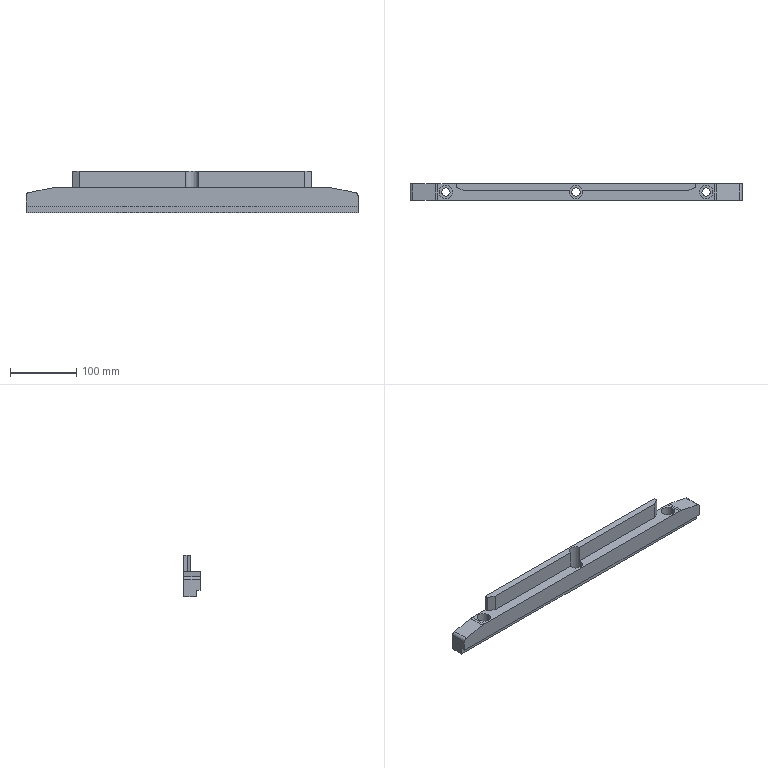NC program | NX | posted with a generic post | part box 500 x 25 x 62.5 mm
Lines 1 to 1034 of 5890:
N10 G17 G21 G94 G90
(ADAPTIVE_MILLING , TOOL : D12JING)
N12 T21 M6
N14 G54
N16 G17 G0 G90 X188.999 Y20.604 S9500 M3
N18 G43 Z30. H21
N20 Z-23.849
N22 G94 G1 Z-24.849 F1000.
N24 X186.723 Y19.599 F3000.
N26 G3 X186. Y18.491 R1.224
N28 G2 X189.082 Y12.674 R11.639
N30 X189.893 Y4.779 R39.403
N32 X189.954 Y-9.769 R368.863
N34 X186.791 Y-14.661 R7.16
N36 X180.65 Y-16.914 R14.438
N38 X172.048 Y-17.442 R63.898
N40 G1 X170.998 Y-17.454
N42 X169.798 Y-17.465
N44 X168.298 Y-17.473
N46 X166.348 Y-17.48
N48 X163.573 Y-17.484
N50 X158.623 Y-17.487
N52 X129.898 Y-17.488
N54 X21.673
N56 X20.923 Y-17.492
N58 X20.023 Y-17.493
N60 X19.573
N62 X18.748 Y-17.496
N64 X17.548 Y-17.495
N66 X16.873 Y-17.497
N68 X15.673 Y-17.496
N70 X14.698 Y-17.499
N72 X13.948 Y-17.498
N74 X12.598 Y-17.5
N76 X12.148 Y-17.501
N78 X11.323 Y-17.499
N80 X10.198 Y-17.501
N82 X9.448 Y-17.499
N84 X8.248 Y-17.501
N86 X7.348 Y-17.499
N88 X6.598 Y-17.5
N90 X5.323 Y-17.498
N92 X4.873
N94 X4.048 Y-17.5
N96 X2.923 Y-17.498
N98 X2.173 Y-17.499
N100 X0.898 Y-17.498
N102 X0.148 Y-17.499
N104 X-1.202 Y-17.497
N106 X-1.877 Y-17.498
N108 X-3.152 Y-17.497
N110 X-3.677
N112 X-4.502 Y-17.499
N114 X-5.702 Y-17.497
N116 X-6.602 Y-17.5
N118 X-7.652 Y-17.497
N120 X-8.477 Y-17.499
N122 X-9.677 Y-17.498
N124 X-10.652 Y-17.5
N126 X-11.627 Y-17.498
N128 X-12.452 Y-17.5
N130 X-13.652 Y-17.498
N132 X-14.327 Y-17.499
N134 X-15.527 Y-17.498
N136 X-16.577 Y-17.501
N138 X-17.477 Y-17.499
N140 X-18.602 Y-17.501
N142 X-19.352 Y-17.499
N144 X-20.552 Y-17.501
N146 X-21.452 Y-17.499
N148 X-22.202 Y-17.5
N150 X-23.477 Y-17.498
N152 X-24.002 Y-17.497
N154 X-24.752 Y-17.499
N156 X-25.952 Y-17.498
N158 X-26.927 Y-17.5
N160 X-27.901 Y-17.498
N162 X-28.726 Y-17.5
N164 X-29.926 Y-17.498
N166 X-30.601 Y-17.499
N168 X-31.801 Y-17.498
N170 X-32.851 Y-17.501
N172 X-33.751 Y-17.499
N174 X-34.876 Y-17.501
N176 X-35.626 Y-17.499
N178 X-36.826 Y-17.501
N180 X-37.726 Y-17.499
N182 X-38.476 Y-17.5
N184 X-39.751 Y-17.498
N186 X-40.276 Y-17.497
N188 X-41.026 Y-17.499
N190 X-42.226 Y-17.498
N192 X-43.201 Y-17.5
N194 X-44.176 Y-17.498
N196 X-45.001 Y-17.5
N198 X-46.201 Y-17.498
N200 X-46.876 Y-17.499
N202 X-48.076 Y-17.498
N204 X-49.126 Y-17.501
N206 X-50.026 Y-17.499
N208 X-51.151 Y-17.501
N210 X-51.901 Y-17.499
N212 X-53.101 Y-17.501
N214 X-54.001 Y-17.499
N216 X-54.751 Y-17.5
N218 X-56.026 Y-17.498
N220 X-56.551 Y-17.497
N222 X-57.301 Y-17.499
N224 X-58.501 Y-17.498
N226 X-59.176 Y-17.499
N228 X-60.301 Y-17.498
N230 X-61.426 Y-17.5
N232 X-62.626 Y-17.497
N234 X-63.301 Y-17.499
N236 X-64.576 Y-17.498
N238 X-65.026 Y-17.497
N240 X-65.776 Y-17.499
N242 X-66.751 Y-17.498
N244 X-67.576 Y-17.5
N246 X-68.701 Y-17.498
N248 X-69.601 Y-17.5
N250 X-70.651 Y-17.498
N252 X-71.326 Y-17.499
N254 X-72.301 Y-17.498
N256 X-72.676
N258 X-73.351 Y-17.499
N260 X-74.401 Y-17.498
N262 X-74.926
N264 X-75.451 Y-17.499
N266 X-76.351 Y-17.498
N268 X-76.726 Y-17.497
N270 X-77.401 Y-17.499
N272 X-78.451 Y-17.498
N274 X-78.901 Y-17.497
N276 X-79.576 Y-17.499
N278 X-80.551 Y-17.498
N280 X-81.076
N282 X-81.751 Y-17.499
N284 X-82.801 Y-17.497
N286 X-83.776 Y-17.5
N288 X-84.676 Y-17.498
N290 X-85.501 Y-17.5
N292 X-86.476 Y-17.498
N294 X-87.301 Y-17.5
N296 X-88.276 Y-17.499
N298 X-88.951 Y-17.5
N300 X-90.226 Y-17.498
N302 X-91.051 Y-17.5
N304 X-92.101 Y-17.498
N306 X-93.076 Y-17.501
N308 X-94.051 Y-17.499
N310 X-94.876 Y-17.5
N312 X-96.076 Y-17.498
N314 X-96.826 Y-17.5
N316 X-97.801 Y-17.499
N318 X-98.851 Y-17.501
N320 X-99.676 Y-17.499
N322 X-100.801 Y-17.501
N324 X-101.626 Y-17.499
N326 X-102.751 Y-17.501
N328 X-103.576 Y-17.499
N330 X-104.476 Y-17.5
N332 X-105.526 Y-17.499
N334 X-106.426 Y-17.501
N336 X-107.476 Y-17.498
N338 X-108.301 Y-17.5
N340 X-109.426 Y-17.498
N342 X-110.176 Y-17.5
N344 X-111.226 Y-17.498
N346 X-112.201 Y-17.5
N348 X-112.876 Y-17.499
N350 X-114.151 Y-17.501
N352 X-114.601 Y-17.502
N354 X-115.351 Y-17.5
N356 X-116.551 Y-17.501
N358 X-117.526 Y-17.499
N360 X-118.501 Y-17.501
N362 X-119.326 Y-17.499
N364 X-120.526 Y-17.501
N366 X-121.201 Y-17.5
N368 X-122.401 Y-17.501
N370 X-123.151 Y-17.5
N372 X-124.351 Y-17.501
N374 X-125.026 Y-17.5
N376 X-126.001 Y-17.501
N378 X-126.451 Y-17.502
N380 X-127.276 Y-17.5
N382 X-128.176 Y-17.501
N384 X-129.001 Y-17.5
N386 X-130.201 Y-17.501
N388 X-130.951 Y-17.5
N390 X-131.926 Y-17.501
N392 X-132.751 Y-17.499
N394 X-133.876 Y-17.501
N396 X-134.701 Y-17.499
N398 X-135.676 Y-17.501
N400 X-136.501 Y-17.499
N402 X-137.551 Y-17.501
N404 X-138.451 Y-17.499
N406 X-139.501 Y-17.501
N408 X-140.326 Y-17.499
N410 X-141.526 Y-17.501
N412 X-142.576 Y-17.498
N414 X-143.401 Y-17.5
N416 X-144.601 Y-17.498
N418 X-145.576 Y-17.501
N420 X-146.476 Y-17.499
N422 X-147.676 Y-17.501
N424 X-148.576 Y-17.499
N426 X-149.551 Y-17.501
N428 X-150.526 Y-17.499
N430 X-151.576 Y-17.501
N432 X-152.401 Y-17.499
N434 X-153.526 Y-17.501
N436 X-154.351 Y-17.499
N438 X-155.476 Y-17.501
N440 X-156.301 Y-17.499
N442 X-157.201 Y-17.5
N444 X-158.026 Y-17.499
N446 X-159.151 Y-17.501
N448 X-160.051 Y-17.499
N450 X-160.951 Y-17.501
N452 X-161.776 Y-17.499
N454 X-162.751 Y-17.5
N456 X-163.801 Y-17.498
N458 X-164.701 Y-17.5
N460 X-165.601 Y-17.499
N462 X-166.501 Y-17.5
N464 X-167.476 Y-17.498
N466 X-168.151 Y-17.499
N468 X-169.426 Y-17.498
N470 X-169.951
N472 X-170.551 Y-17.499
N474 X-171.526 Y-17.498
N476 X-172.276 Y-17.5
N478 X-173.326 Y-17.498
N480 X-174.301 Y-17.5
N482 X-174.976 Y-17.499
N484 X-176.251 Y-17.501
N486 X-176.776
N488 G2 X-182.25 Y-17.469 R279.255
N490 X-187.15 Y-14.319 R7.147
N492 X-189.421 Y-8.106 R14.464
N494 X-189.954 Y1.471 R71.167
N496 X-189.956 Y9.795 R359.357
N498 X-187.917 Y14.399 R9.324
N500 G3 X-186.115 Y16.886 R22.32
N502 G1 X-186.089 Y16.956
N504 X-186.067 Y17.028
N506 X-186.048 Y17.1
N508 X-186.034 Y17.174
N510 X-186.024 Y17.248
N512 X-186.328 Y18.409
N514 G3 X-187.009 Y19.204 R1.217
N516 X-188.412 Y18.879 Z-24.785 R1.228
N518 G1 X-189.02 Y18.273 Z-24.749
N520 X-189.418 Y17.87
N522 X-189.833 Y17.485
N524 G2 X-191.728 Y18.409 R1.202
N526 G1 X-191.757 Y18.961
N528 X-191.76 Y19.514
N530 G2 X-190.268 Y20.526 R1.204
N532 G1 X-189.229 Y20.257
N534 X-186.906 Y19.653 Z-24.849
N536 G2 X-186.368 Y19.311 R1.26
N538 X-186.018 Y18.462 R1.291
N540 X-186.092 Y16.745 R6.843
N542 X-187.495 Y14.099 R19.023
N544 G3 X-189.115 Y7.901 R16.064
N546 X-188.942 Y-6.48 R85.448
N548 X-187.347 Y-11.993 R14.997
N550 X-182.305 Y-15.789 R8.996
N552 X-175.501 Y-16.787 R24.761
N554 X-155.402 Y-16.9 R819.463
N556 G1 X-153.827 Y-16.902
N558 X-153.152
N560 X-152.777 Y-16.901
N562 X-151.877 Y-16.902
N564 X-151.277 Y-16.9
N566 X-150.002 Y-16.902
N568 X-149.327 Y-16.9
N570 X-147.752 Y-16.902
N572 X-146.777 Y-16.9
N574 X-146.102 Y-16.901
N576 X-144.977 Y-16.899
N578 X-144.152 Y-16.901
N580 X-142.652 Y-16.898
N582 X-141.902 Y-16.9
N584 X-141.152 Y-16.898
N586 X-139.577 Y-16.901
N588 X-139.127
N590 X-138.002 Y-16.902
N592 X-137.477 Y-16.901
N594 X-136.427 Y-16.899
N596 X-135.977 Y-16.9
N598 X-135.602 Y-16.899
N600 X-134.102 Y-16.902
N602 X-133.577
N604 X-132.452 Y-16.903
N606 X-131.927 Y-16.902
N608 X-128.852 Y-16.898
N610 X-126.377
N612 X-124.352 Y-16.901
N614 X-123.827
N616 X-122.852 Y-16.903
N618 X-122.327 Y-16.901
N620 X-120.602 Y-16.903
N622 X-120.152 Y-16.902
N624 X-118.727 Y-16.904
N626 X-118.277 Y-16.903
N628 X-117.902
N630 X-117.602 Y-16.902
N632 X-116.852 Y-16.903
N634 X-116.327 Y-16.902
N636 X-115.502 Y-16.903
N638 X-114.902 Y-16.902
N640 X-114.452
N642 X-113.777 Y-16.9
N644 X-113.027 Y-16.901
N646 X-111.902 Y-16.898
N648 X-110.477 Y-16.901
N650 X-110.027 Y-16.9
N652 X-108.827 Y-16.902
N654 X-108.152 Y-16.9
N656 X-107.177 Y-16.901
N658 X-106.127 Y-16.899
N660 X-105.527 Y-16.9
N662 X-104.027 Y-16.898
N664 X-103.127 Y-16.9
N666 X-102.002 Y-16.898
N668 X-101.252 Y-16.9
N670 X-100.652 Y-16.899
N672 X-99.602 Y-16.901
N674 X-98.402 Y-16.898
N676 X-97.877 Y-16.899
N678 X-96.452 Y-16.897
N680 X-95.477 Y-16.899
N682 X-94.577 Y-16.897
N684 X-94.052 Y-16.898
N686 X-92.327 Y-16.896
N688 X-91.652 Y-16.898
N690 X-90.377 Y-16.896
N692 X-89.777 Y-16.898
N694 X-88.952 Y-16.897
N696 X-87.902 Y-16.899
N698 X-86.852 Y-16.897
N700 X-86.027 Y-16.899
N702 X-85.352 Y-16.897
N704 X-84.602 Y-16.899
N706 X-83.102 Y-16.896
N708 X-82.202 Y-16.899
N710 X-81.602 Y-16.897
N712 X-80.027 Y-16.9
N714 X-79.052 Y-16.898
N716 X-77.627 Y-16.9
N718 X-77.102 Y-16.899
N720 X-76.352 Y-16.901
N722 X-75.153 Y-16.898
N724 X-74.628 Y-16.899
N726 X-74.028 Y-16.897
N728 X-73.503 Y-16.898
N730 X-72.828 Y-16.897
N732 X-72.003 Y-16.899
N734 X-71.328 Y-16.898
N736 X-69.753 Y-16.9
N738 X-69.303 Y-16.899
N740 X-68.553 Y-16.901
N742 X-67.278 Y-16.898
N744 X-65.703 Y-16.9
N746 X-65.253 Y-16.899
N748 X-64.128 Y-16.901
N750 X-62.853 Y-16.898
N752 X-61.503 Y-16.9
N754 X-60.978 Y-16.899
N756 X-60.303 Y-16.9
N758 X-59.853 Y-16.899
N760 X-59.478 Y-16.9
N762 X-58.878 Y-16.899
N764 X-57.678 Y-16.901
N766 X-56.628 Y-16.898
N768 X-55.878 Y-16.9
N770 X-54.303 Y-16.898
N772 X-53.478 Y-16.9
N774 X-52.278 Y-16.898
N776 X-51.528 Y-16.9
N778 X-50.628 Y-16.898
N780 X-49.203 Y-16.9
N782 X-48.753
N784 X-47.853 Y-16.901
N786 X-46.653 Y-16.898
N788 X-45.828 Y-16.9
N790 X-45.003 Y-16.898
N792 X-43.353 Y-16.901
N794 X-42.903 Y-16.899
N796 X-41.778 Y-16.901
N798 X-41.328 Y-16.9
N800 X-40.578 Y-16.901
N802 X-39.153 Y-16.903
N804 X-38.628 Y-16.901
N806 X-37.803 Y-16.9
N808 X-37.353
N810 X-36.678 Y-16.899
N812 X-35.328 Y-16.902
N814 X-34.578 Y-16.899
N816 X-32.853 Y-16.902
N818 X-32.403 Y-16.901
N820 X-31.128 Y-16.902
N822 X-30.678 Y-16.901
N824 X-29.928 Y-16.9
N826 X-29.328 Y-16.901
N828 X-28.653 Y-16.899
N830 X-27.003 Y-16.901
N832 X-26.103 Y-16.899
N834 X-25.428 Y-16.9
N836 X-24.903 Y-16.899
N838 X-24.303 Y-16.9
N840 X-22.878 Y-16.902
N842 X-22.503 Y-16.901
N844 X-21.828 Y-16.902
N846 X-21.378 Y-16.901
N848 X-20.928 Y-16.902
N850 X-20.253 Y-16.9
N852 X-18.678 Y-16.902
N854 X-16.878 Y-16.903
N856 X-15.903 Y-16.9
N858 X-15.003 Y-16.902
N860 X-13.803 Y-16.899
N862 X-13.053 Y-16.9
N864 X-12.078 Y-16.898
N866 X-11.403 Y-16.9
N868 X-10.053 Y-16.897
N870 X-9.528 Y-16.898
N872 X-7.728 Y-16.895
N874 X-6.903 Y-16.898
N876 X-6.078 Y-16.896
N878 X-4.653 Y-16.899
N880 X-3.528 Y-16.897
N882 X-2.103 Y-16.9
N884 X-1.428 Y-16.898
N886 X-0.828 Y-16.899
N888 X0.522 Y-16.897
N890 X1.797 Y-16.899
N892 X2.397 Y-16.898
N894 X3.147 Y-16.9
N896 X3.597 Y-16.899
N898 X4.347 Y-16.9
N900 X4.797
N902 X5.922 Y-16.902
N904 X6.597 Y-16.9
N906 X8.097 Y-16.902
N908 X9.897 Y-16.904
N910 X11.097 Y-16.9
N912 X12.372 Y-16.902
N914 X12.897 Y-16.901
N916 X13.647 Y-16.899
N918 X14.022 Y-16.9
N920 X15.372 Y-16.896
N922 X15.897 Y-16.897
N924 X18.072 Y-16.892
N926 X18.672 Y-16.893
N928 X19.497 Y-16.89
N930 X20.997 Y-16.892
N932 X21.522 Y-16.89
N934 X23.022 Y-16.892
N936 X23.622 Y-16.89
N938 X24.522 Y-16.888
N940 X25.347 Y-16.89
N942 X26.022 Y-16.888
N944 X26.847 Y-16.89
N946 X27.447 Y-16.888
N948 X28.272 Y-16.89
N950 X28.872 Y-16.888
N952 X29.622 Y-16.89
N954 X30.222 Y-16.888
N956 X31.047 Y-16.89
N958 X31.647 Y-16.888
N960 X32.397 Y-16.89
N962 X32.997 Y-16.888
N964 X33.822 Y-16.89
N966 X34.422 Y-16.888
N968 X35.172 Y-16.89
N970 X35.772 Y-16.888
N972 X36.597 Y-16.89
N974 X37.197 Y-16.888
N976 X37.947 Y-16.89
N978 X38.547 Y-16.888
N980 X39.372 Y-16.89
N982 X40.047 Y-16.888
N984 X40.872 Y-16.89
N986 X41.472 Y-16.888
N988 X42.297 Y-16.89
N990 X42.897 Y-16.888
N992 X43.647 Y-16.89
N994 X44.247 Y-16.888
N996 X45.072 Y-16.89
N998 X45.672 Y-16.888
N1000 X46.422 Y-16.89
N1002 X47.022 Y-16.888
N1004 X47.847 Y-16.89
N1006 X48.447 Y-16.888
N1008 X49.197 Y-16.89
N1010 X49.797 Y-16.888
N1012 X50.622 Y-16.89
N1014 X51.222 Y-16.888
N1016 X51.972 Y-16.89
N1018 X52.572 Y-16.888
N1020 X53.397 Y-16.89
N1022 X53.997 Y-16.888
N1024 X54.747 Y-16.89
N1026 X55.347 Y-16.888
N1028 X56.172 Y-16.89
N1030 X56.847 Y-16.888
N1032 X57.672 Y-16.89
N1034 X58.272 Y-16.888
N1036 X59.097 Y-16.89
N1038 X59.697 Y-16.888
N1040 X60.447 Y-16.89
N1042 X61.047 Y-16.888
N1044 X61.872 Y-16.89
N1046 X62.472 Y-16.888
N1048 X63.222 Y-16.89
N1050 X63.822 Y-16.888
N1052 X64.647 Y-16.89
N1054 X65.247 Y-16.888
N1056 X65.997 Y-16.89
N1058 X66.597 Y-16.888
N1060 X67.422 Y-16.89
N1062 X68.022 Y-16.888
N1064 X68.772 Y-16.89
N1066 X69.372 Y-16.888
N1068 X70.197 Y-16.89
N1070 X70.797 Y-16.888
N1072 X71.547 Y-16.89
N1074 X72.147 Y-16.888
N1076 X72.972 Y-16.89
N1078 X73.647 Y-16.888
N1080 X74.472 Y-16.89
N1082 X75.072 Y-16.888
N1084 X75.897 Y-16.89
N1086 X76.497 Y-16.888
N1088 X77.247 Y-16.89
N1090 X77.847 Y-16.888
N1092 X78.672 Y-16.89
N1094 X79.272 Y-16.888
N1096 X80.022 Y-16.89
N1098 X80.622 Y-16.888
N1100 X81.447 Y-16.89
N1102 X82.047 Y-16.888
N1104 X82.797 Y-16.89
N1106 X83.397 Y-16.888
N1108 X84.222 Y-16.89
N1110 X84.897 Y-16.888
N1112 X85.797 Y-16.89
N1114 X86.472 Y-16.888
N1116 X87.297 Y-16.89
N1118 X87.897 Y-16.888
N1120 X88.722 Y-16.89
N1122 X89.397 Y-16.888
N1124 X90.297 Y-16.89
N1126 X90.972 Y-16.888
N1128 X91.797 Y-16.89
N1130 X92.397 Y-16.888
N1132 X93.222 Y-16.89
N1134 X93.897 Y-16.888
N1136 X94.797 Y-16.89
N1138 X95.472 Y-16.888
N1140 X96.297 Y-16.89
N1142 X96.897 Y-16.888
N1144 X97.722 Y-16.89
N1146 X98.397 Y-16.888
N1148 X99.297 Y-16.89
N1150 X99.972 Y-16.888
N1152 X100.797 Y-16.89
N1154 X101.397 Y-16.888
N1156 X102.222 Y-16.89
N1158 X102.897 Y-16.888
N1160 X103.797 Y-16.89
N1162 X104.472 Y-16.888
N1164 X105.297 Y-16.89
N1166 X105.897 Y-16.888
N1168 X106.722 Y-16.89
N1170 X107.397 Y-16.888
N1172 X108.297 Y-16.89
N1174 X108.972 Y-16.888
N1176 X109.797 Y-16.89
N1178 X110.397 Y-16.888
N1180 X111.222 Y-16.89
N1182 X111.897 Y-16.888
N1184 X112.797 Y-16.89
N1186 X113.472 Y-16.888
N1188 X114.372 Y-16.89
N1190 X115.047 Y-16.888
N1192 X115.872 Y-16.89
N1194 X116.472 Y-16.888
N1196 X117.297 Y-16.89
N1198 X117.972 Y-16.888
N1200 X118.872 Y-16.89
N1202 X119.547 Y-16.888
N1204 X120.372 Y-16.89
N1206 X120.972 Y-16.888
N1208 X121.797 Y-16.89
N1210 X122.472 Y-16.888
N1212 X123.372 Y-16.89
N1214 X124.047 Y-16.888
N1216 X124.872 Y-16.89
N1218 X125.472 Y-16.888
N1220 X126.297 Y-16.89
N1222 X126.972 Y-16.888
N1224 X127.872 Y-16.89
N1226 X128.547 Y-16.888
N1228 X129.372 Y-16.89
N1230 X129.972 Y-16.888
N1232 X130.797 Y-16.89
N1234 X131.472 Y-16.888
N1236 X132.372 Y-16.89
N1238 X133.047 Y-16.888
N1240 X133.872 Y-16.89
N1242 X134.472 Y-16.888
N1244 X135.297 Y-16.89
N1246 X135.972 Y-16.888
N1248 X136.872 Y-16.89
N1250 X137.547 Y-16.888
N1252 X138.372 Y-16.89
N1254 X138.972 Y-16.888
N1256 X139.797 Y-16.89
N1258 X140.472 Y-16.888
N1260 X141.372 Y-16.89
N1262 X142.047 Y-16.888
N1264 X142.872 Y-16.89
N1266 X143.472 Y-16.888
N1268 X144.297 Y-16.89
N1270 X144.972 Y-16.888
N1272 X145.872 Y-16.89
N1274 X146.547 Y-16.888
N1276 X147.372 Y-16.89
N1278 X148.047 Y-16.888
N1280 X148.947 Y-16.89
N1282 X149.622 Y-16.888
N1284 X150.447 Y-16.889
N1286 X151.122 Y-16.888
N1288 X151.947 Y-16.889
N1290 X152.622 Y-16.888
N1292 X153.447 Y-16.889
N1294 X154.122 Y-16.888
N1296 X154.947 Y-16.889
N1298 X155.697 Y-16.887
N1300 X156.447 Y-16.889
N1302 X157.197 Y-16.887
N1304 X157.947 Y-16.888
N1306 X158.772 Y-16.886
N1308 X159.447 Y-16.888
N1310 X160.497 Y-16.885
N1312 X161.097 Y-16.886
N1314 X162.897 Y-16.882
N1316 X163.497
N1318 X164.247
N1320 X165.297 Y-16.881
N1322 X166.422 Y-16.88
N1324 G3 X177.814 Y-16.568 R149.249
N1326 X183.919 Y-15.143 R18.297
N1328 X188.11 Y-10.259 R8.557
N1330 X189.221 Y-3.931 R21.167
N1332 X188.969 Y9.106 R92.609
N1334 X186.487 Y16.423 R16.369
N1336 G2 X186.01 Y17.518 R4.405
N1338 G1 X186.364 Y18.664
N1340 G2 X186.969 Y19.381 R1.229
N1342 X188.44 Y19.077 Z-24.782 R1.224
N1344 G1 X188.991 Y18.523 Z-24.749
N1346 X189.42 Y18.084
N1348 X189.868 Y17.664
N1350 G3 X191.764 Y18.664 R1.202
N1352 G1 X191.757 Y19.099
N1354 X191.732 Y19.533
N1356 G3 X190.275 Y20.485 R1.205
N1358 G1 X189.224 Y20.236
N1360 X186.889 Y19.681 Z-24.849
N1362 G3 X186.351 Y19.339 R1.261
N1364 X186. Y18.491 R1.291
N1366 X186.32 Y15.753 R7.183
N1368 G2 X188.191 Y3.713 R43.619
N1370 X187.944 Y-5.498 R56.86
N1372 X185.845 Y-10.795 R10.316
N1374 X179.757 Y-14.575 R12.155
N1376 X171.531 Y-15.709 R34.419
N1378 X151.958 Y-15.885 R599.038
N1380 G1 X150.758 Y-15.884
N1382 X150.158 Y-15.886
N1384 X148.958
N1386 X148.208 Y-15.884
N1388 X147.383 Y-15.887
N1390 X146.258 Y-15.886
N1392 X145.358 Y-15.888
N1394 X144.608 Y-15.887
N1396 X143.183 Y-15.891
N1398 X142.133 Y-15.888
N1400 X141.233 Y-15.889
N1402 X140.258 Y-15.888
N1404 X139.508 Y-15.889
N1406 X138.758 Y-15.888
N1408 X138.158 Y-15.887
N1410 X137.033 Y-15.89
N1412 X136.133 Y-15.888
N1414 X135.008 Y-15.89
N1416 X134.108 Y-15.888
N1418 X133.208 Y-15.89
N1420 X132.308 Y-15.888
N1422 X131.033 Y-15.891
N1424 X130.058 Y-15.888
N1426 X129.158 Y-15.89
N1428 X127.958 Y-15.888
N1430 X127.283 Y-15.889
N1432 X126.008 Y-15.887
N1434 X124.958 Y-15.89
N1436 X123.908 Y-15.888
N1438 X123.158 Y-15.889
N1440 X121.958 Y-15.888
N1442 X121.433
N1444 X120.458 Y-15.891
N1446 X119.483 Y-15.888
N1448 X118.658 Y-15.89
N1450 X117.533 Y-15.888
N1452 X116.933 Y-15.889
N1454 X115.733 Y-15.887
N1456 X115.283
N1458 X114.383 Y-15.89
N1460 X113.408 Y-15.888
N1462 X112.358 Y-15.89
N1464 X111.533 Y-15.888
N1466 X110.483 Y-15.89
N1468 X109.433 Y-15.887
N1470 X108.458 Y-15.89
N1472 X107.408 Y-15.888
N1474 X106.508 Y-15.889
N1476 X105.608 Y-15.888
N1478 X104.708 Y-15.89
N1480 X103.583 Y-15.887
N1482 X102.458 Y-15.89
N1484 X101.633 Y-15.888
N1486 X100.658 Y-15.89
N1488 X100.133
N1490 X99.533 Y-15.889
N1492 X98.483 Y-15.89
N1494 X97.133 Y-15.887
N1496 X96.233 Y-15.889
N1498 X95.108 Y-15.887
N1500 X94.358 Y-15.889
N1502 X93.008 Y-15.887
N1504 X91.883 Y-15.89
N1506 X91.133 Y-15.889
N1508 X89.558 Y-15.89
N1510 X88.733 Y-15.891
N1512 X87.908 Y-15.889
N1514 X86.858 Y-15.89
N1516 X86.033 Y-15.889
N1518 X84.608 Y-15.892
N1520 X83.633 Y-15.889
N1522 X82.658 Y-15.891
N1524 X81.983 Y-15.889
N1526 X80.933 Y-15.891
N1528 X80.408
N1530 X79.433 Y-15.889
N1532 X78.683 Y-15.89
N1534 X77.483 Y-15.888
N1536 X76.958 Y-15.887
N1538 X76.058 Y-15.889
N1540 X75.158 Y-15.888
N1542 X74.108 Y-15.889
N1544 X72.683 Y-15.886
N1546 X71.933 Y-15.888
N1548 X70.808 Y-15.887
N1550 X70.283
N1552 X69.233 Y-15.89
N1554 X68.408 Y-15.888
N1556 X67.208 Y-15.89
N1558 X66.458 Y-15.888
N1560 X65.708 Y-15.889
N1562 X65.033 Y-15.891
N1564 X64.133 Y-15.889
N1566 X63.008 Y-15.89
N1568 X62.258 Y-15.889
N1570 X61.358 Y-15.891
N1572 X60.833
N1574 X59.933 Y-15.889
N1576 X58.958 Y-15.89
N1578 X58.133 Y-15.889
N1580 X57.158 Y-15.89
N1582 X56.108 Y-15.887
N1584 X54.983 Y-15.89
N1586 X54.083 Y-15.888
N1588 X53.108 Y-15.89
N1590 X52.433 Y-15.889
N1592 X51.533 Y-15.89
N1594 X51.008 Y-15.891
N1596 X50.108 Y-15.889
N1598 X49.133 Y-15.89
N1600 X48.308 Y-15.889
N1602 X46.808 Y-15.892
N1604 X45.983 Y-15.89
N1606 X44.858
N1608 X44.033 Y-15.889
N1610 X43.358 Y-15.89
N1612 X42.533 Y-15.888
N1614 X41.933 Y-15.887
N1616 X40.958 Y-15.89
N1618 X40.058 Y-15.888
N1620 X38.933 Y-15.89
N1622 X38.333 Y-15.889
N1624 X37.133 Y-15.89
N1626 X36.758 Y-15.891
N1628 X36.008 Y-15.889
N1630 X34.808 Y-15.89
N1632 X33.833 Y-15.888
N1634 X32.708 Y-15.891
N1636 X31.958 Y-15.889
N1638 X30.758 Y-15.89
N1640 X30.008 Y-15.892
N1642 X29.033 Y-15.889
N1644 X27.983 Y-15.891
N1646 X27.233 Y-15.89
N1648 X26.108 Y-15.891
N1650 X25.658
N1652 X24.908 Y-15.89
N1654 X24.008 Y-15.892
N1656 X23.633
N1658 X22.583 Y-15.89
N1660 X21.683 Y-15.892
N1662 X20.633 Y-15.891
N1664 X19.358 Y-15.895
N1666 X18.383 Y-15.893
N1668 X17.108 Y-15.898
N1670 X16.358 Y-15.897
N1672 X15.158 Y-15.899
N1674 X14.033 Y-15.898
N1676 X13.283 Y-15.9
N1678 X12.008 Y-15.899
N1680 X11.483
N1682 X10.808 Y-15.901
N1684 X9.758 Y-15.899
N1686 X9.233 Y-15.9
N1688 X8.558 Y-15.901
N1690 X7.508 Y-15.899
N1692 X6.383 Y-15.902
N1694 X5.408 Y-15.899
N1696 X4.583 Y-15.9
N1698 X3.308 Y-15.898
N1700 X2.858 Y-15.897
N1702 X1.958 Y-15.899
N1704 X0.983 Y-15.898
N1706 X0.233 Y-15.899
N1708 X-0.817 Y-15.897
N1710 X-1.867 Y-15.899
N1712 X-2.992 Y-15.896
N1714 X-3.967 Y-15.898
N1716 X-4.867 Y-15.896
N1718 X-5.917 Y-15.897
N1720 X-6.967 Y-15.896
N1722 X-8.167 Y-15.899
N1724 X-9.067 Y-15.897
N1726 X-10.192 Y-15.899
N1728 X-11.092 Y-15.898
N1730 X-12.067 Y-15.9
N1732 X-13.117 Y-15.899
N1734 X-14.167 Y-15.901
N1736 X-15.067 Y-15.9
N1738 X-15.967 Y-15.902
N1740 X-17.092 Y-15.9
N1742 X-17.992 Y-15.901
N1744 X-19.042 Y-15.9
N1746 X-20.017 Y-15.903
N1748 X-21.142 Y-15.9
N1750 X-22.267 Y-15.903
N1752 X-23.017 Y-15.901
N1754 X-24.217
N1756 X-24.742 Y-15.902
N1758 X-25.567 Y-15.9
N1760 X-26.692 Y-15.902
N1762 X-27.667 Y-15.899
N1764 X-28.492 Y-15.901
N1766 X-29.617 Y-15.9
N1768 X-30.517 Y-15.902
N1770 X-31.642 Y-15.899
N1772 X-32.392 Y-15.901
N1774 X-33.442 Y-15.899
N1776 X-33.892
N1778 X-34.717 Y-15.9
N1780 X-35.542 Y-15.899
N1782 X-36.517 Y-15.901
N1784 X-37.792 Y-15.899
N1786 X-38.692 Y-15.901
N1788 X-39.817 Y-15.899
N1790 X-40.717 Y-15.901
N1792 X-41.842 Y-15.898
N1794 X-42.742 Y-15.9
N1796 X-43.717 Y-15.899
N1798 X-44.842 Y-15.901
N1800 X-45.892 Y-15.899
N1802 X-46.717 Y-15.9
N1804 X-47.692 Y-15.899
N1806 X-48.667 Y-15.9
N1808 X-49.567 Y-15.898
N1810 X-50.467 Y-15.9
N1812 X-51.517 Y-15.898
N1814 X-52.642 Y-15.9
N1816 X-53.617 Y-15.898
N1818 X-54.517 Y-15.9
N1820 X-55.342 Y-15.899
N1822 X-55.792 Y-15.898
N1824 X-56.617 Y-15.899
N1826 X-57.742 Y-15.898
N1828 X-58.567 Y-15.9
N1830 X-59.467 Y-15.898
N1832 X-59.842
N1834 X-61.042 Y-15.9
N1836 X-62.167 Y-15.898
N1838 X-63.142 Y-15.9
N1840 X-64.192 Y-15.898
N1842 X-65.392 Y-15.9
N1844 X-66.142 Y-15.899
N1846 X-67.342 Y-15.901
N1848 X-68.392 Y-15.898
N1850 X-69.142 Y-15.899
N1852 X-70.342 Y-15.897
N1854 X-70.867 Y-15.896
N1856 X-71.617 Y-15.897
N1858 X-73.117
N1860 X-74.017 Y-15.895
N1862 X-74.692 Y-15.897
N1864 X-75.967
N1866 X-76.642 Y-15.896
N1868 X-77.242 Y-15.898
N1870 X-78.517 Y-15.897
N1872 X-79.042 Y-15.896
N1874 X-79.642 Y-15.897
N1876 X-80.917 Y-15.896
N1878 X-81.742 Y-15.898
N1880 X-82.867 Y-15.897
N1882 X-83.542 Y-15.898
N1884 X-84.442 Y-15.897
N1886 X-85.042 Y-15.896
N1888 X-85.792 Y-15.897
N1890 X-86.617 Y-15.896
N1892 X-87.217 Y-15.895
N1894 X-88.192 Y-15.897
N1896 X-89.242 Y-15.895
N1898 X-90.367 Y-15.898
N1900 X-91.042 Y-15.897
N1902 X-92.092 Y-15.898
N1904 X-92.617 Y-15.899
N1906 X-93.292 Y-15.898
N1908 X-94.192 Y-15.899
N1910 X-94.792 Y-15.9
N1912 X-95.617 Y-15.898
N1914 X-96.742 Y-15.9
N1916 X-97.867 Y-15.898
N1918 X-98.542 Y-15.899
N1920 X-99.816 Y-15.898
N1922 X-100.566 Y-15.899
N1924 X-101.541 Y-15.898
N1926 X-102.441 Y-15.9
N1928 X-103.566 Y-15.898
N1930 X-104.316 Y-15.9
N1932 X-105.441 Y-15.899
N1934 X-106.116 Y-15.898
N1936 X-106.791 Y-15.899
N1938 X-107.916 Y-15.898
N1940 X-108.741 Y-15.896
N1942 X-109.941 Y-15.9
N1944 X-110.766 Y-15.899
N1946 X-111.966 Y-15.901
N1948 X-112.566 Y-15.902
N1950 X-113.316 Y-15.901
N1952 X-114.216 Y-15.902
N1954 X-114.816 Y-15.904
N1956 X-115.641 Y-15.902
N1958 X-116.766 Y-15.905
N1960 X-117.666 Y-15.903
N1962 X-118.641 Y-15.904
N1964 X-119.391 Y-15.903
N1966 X-120.516 Y-15.904
N1968 X-121.191 Y-15.903
N1970 X-121.716 Y-15.901
N1972 X-122.391 Y-15.902
N1974 X-123.366 Y-15.9
N1976 X-123.816 Y-15.899
N1978 X-124.566 Y-15.9
N1980 X-125.691 Y-15.898
N1982 X-126.516 Y-15.899
N1984 X-127.566 Y-15.898
N1986 X-128.691 Y-15.901
N1988 X-129.366
N1990 X-130.866 Y-15.903
N1992 X-131.466 Y-15.902
N1994 X-132.216 Y-15.9
N1996 X-133.191 Y-15.902
N1998 X-133.941 Y-15.9
N2000 X-134.841 Y-15.902
N2002 X-135.366
N2004 X-136.266 Y-15.9
N2006 X-137.016 Y-15.901
N2008 X-138.141 Y-15.899
N2010 X-138.591
N2012 X-139.191 Y-15.9
N2014 X-140.466 Y-15.898
N2016 X-141.291 Y-15.9
N2018 X-142.341 Y-15.898
N2020 X-143.166 Y-15.9
N2022 X-144.216 Y-15.899
N2024 X-145.041 Y-15.901
N2026 X-146.241 Y-15.899
N2028 X-147.141 Y-15.901
N2030 X-148.191 Y-15.9
N2032 X-149.091 Y-15.901
N2034 X-150.216 Y-15.9
N2036 X-151.041 Y-15.902
N2038 X-151.716 Y-15.901
N2040 X-152.316 Y-15.9
N2042 X-153.066 Y-15.901
N2044 X-154.191 Y-15.9
N2046 X-155.016 Y-15.902
N2048 G2 X-174.29 Y-15.784 R776.226
N2050 X-180.58 Y-14.883 R22.809
N2052 X-186.102 Y-9.77 R9.815
N2054 X-187.967 Y-2.395 R21.071
N2056 X-187.907 Y8.159 R48.463
N2058 X-186.329 Y13.387 R22.351
N2060 G3 X-186.023 Y14.342 R5.41
N2062 G1 X-186.02 Y17.117
N2064 X-186.023 Y14.342
N2066 G2 X-186.536 Y11.546 R12.342